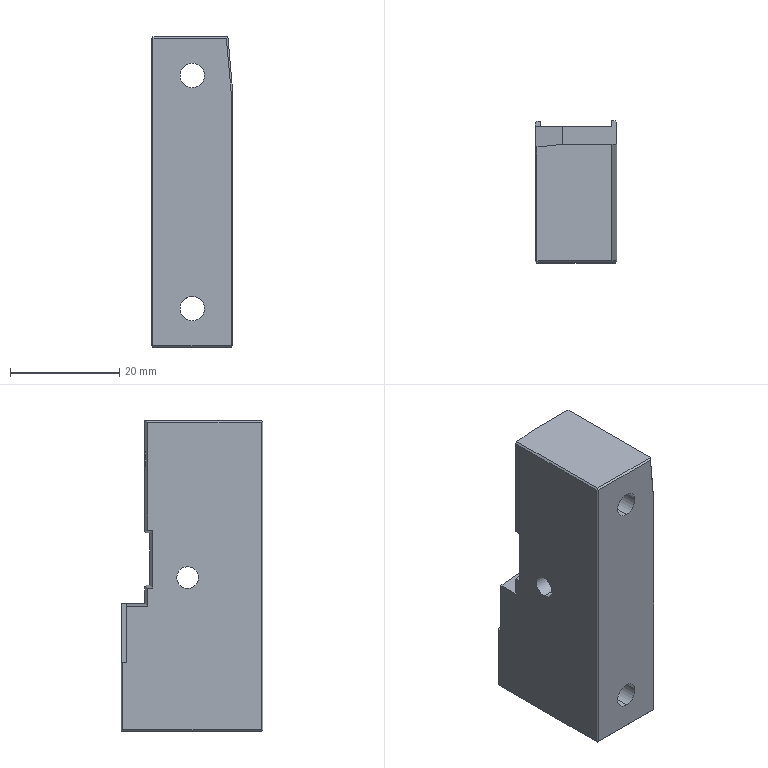Part | NX | 1 solid | 62 faces | box 14.9 x 26 x 57 mm | volume 17731 mm3 | plane 38 | cylinder 18 | cone 6 | commonest cylinder face diameters 8 x6 3.3 x4 4.5 x4 2.5 x2 4 x2